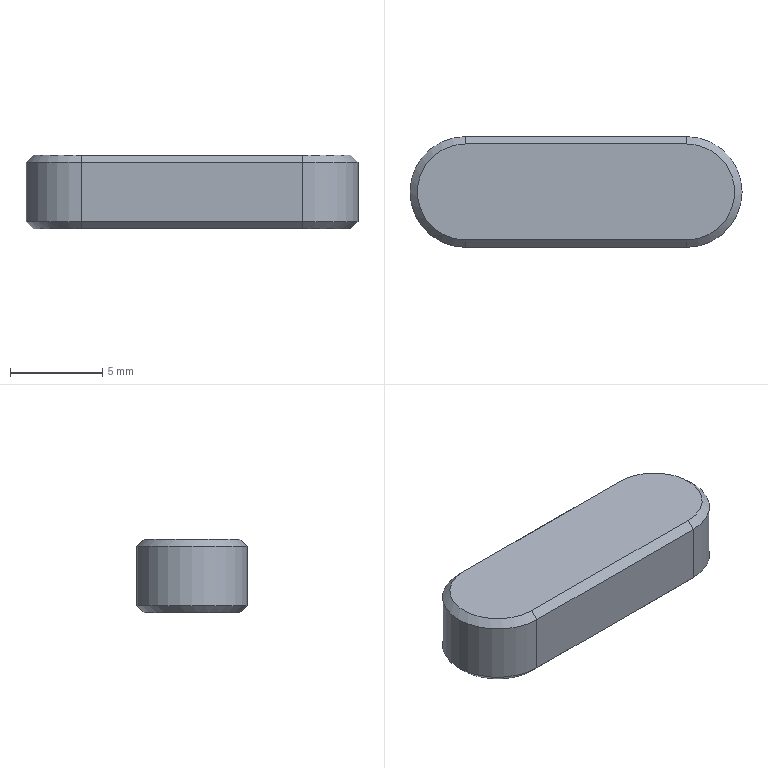Part | SolidWorks | features BaseBody 1 | 1 solid | 14 faces | box 18 x 6 x 4 mm | volume 394.375 mm3 | plane 8 | cone 4 | cylinder 2 | commonest cylinder face diameters 6 x2
STEP:
#1=CARTESIAN_POINT('',(15.,-2.6,-2.5));
#2=VERTEX_POINT('',#1);
#3=CARTESIAN_POINT('',(15.,-3.,-2.1));
#4=VERTEX_POINT('',#3);
#5=CARTESIAN_POINT('',(15.,-2.6,-2.5));
#6=DIRECTION('',(0.,-0.7071,0.7071));
#7=VECTOR('',#6,1000.);
#8=LINE('',#5,#7);
#9=EDGE_CURVE('',#2,#4,#8,.T.);
#10=ORIENTED_EDGE('',*,*,#9,.T.);
#11=CARTESIAN_POINT('',(3.,-3.,-2.1));
#12=VERTEX_POINT('',#11);
#13=CARTESIAN_POINT('',(6.,-3.,-2.1));
#14=DIRECTION('',(-1.,0.,0.));
#15=VECTOR('',#14,1000.);
#16=LINE('',#13,#15);
#17=EDGE_CURVE('',#4,#12,#16,.T.);
#18=ORIENTED_EDGE('',*,*,#17,.T.);
#19=CARTESIAN_POINT('',(3.,-2.6,-2.5));
#20=VERTEX_POINT('',#19);
#21=CARTESIAN_POINT('',(3.,-3.,-2.1));
#22=DIRECTION('',(0.,0.7071,-0.7071));
#23=VECTOR('',#22,1000.);
#24=LINE('',#21,#23);
#25=EDGE_CURVE('',#12,#20,#24,.T.);
#26=ORIENTED_EDGE('',*,*,#25,.T.);
#27=CARTESIAN_POINT('',(6.,-2.6,-2.5));
#28=DIRECTION('',(1.,0.,0.));
#29=VECTOR('',#28,1000.);
#30=LINE('',#27,#29);
#31=EDGE_CURVE('',#20,#2,#30,.T.);
#32=ORIENTED_EDGE('',*,*,#31,.T.);
#33=EDGE_LOOP('',(#10,#18,#26,#32));
#34=FACE_OUTER_BOUND('',#33,.T.);
#35=CARTESIAN_POINT('',(6.,-2.8,-2.3));
#36=DIRECTION('',(0.,-0.7071,-0.7071));
#37=DIRECTION('',(0.,-0.7071,0.7071));
#38=AXIS2_PLACEMENT_3D('',#35,#36,#37);
#39=PLANE('',#38);
#40=ADVANCED_FACE('',(#34),#39,.T.);
#41=CARTESIAN_POINT('',(15.,2.6,-2.5));
#42=VERTEX_POINT('',#41);
#43=CARTESIAN_POINT('',(15.,3.,-2.1));
#44=VERTEX_POINT('',#43);
#45=CARTESIAN_POINT('',(15.,2.6,-2.5));
#46=DIRECTION('',(0.,0.7071,0.7071));
#47=VECTOR('',#46,1000.);
#48=LINE('',#45,#47);
#49=EDGE_CURVE('',#42,#44,#48,.T.);
#50=ORIENTED_EDGE('',*,*,#49,.T.);
#51=CARTESIAN_POINT('',(15.,0.,-2.1));
#52=DIRECTION('',(0.,0.,-1.));
#53=DIRECTION('',(0.,1.,0.));
#54=AXIS2_PLACEMENT_3D('',#51,#52,#53);
#55=CIRCLE('',#54,3.);
#56=EDGE_CURVE('',#44,#4,#55,.T.);
#57=ORIENTED_EDGE('',*,*,#56,.T.);
#58=ORIENTED_EDGE('',*,*,#9,.F.);
#59=CARTESIAN_POINT('',(15.,0.,-2.5));
#60=DIRECTION('',(0.,0.,1.));
#61=DIRECTION('',(0.,1.,0.));
#62=AXIS2_PLACEMENT_3D('',#59,#60,#61);
#63=CIRCLE('',#62,2.6);
#64=EDGE_CURVE('',#2,#42,#63,.T.);
#65=ORIENTED_EDGE('',*,*,#64,.T.);
#66=EDGE_LOOP('',(#50,#57,#58,#65));
#67=FACE_OUTER_BOUND('',#66,.T.);
#68=CARTESIAN_POINT('',(15.,0.,-2.3));
#69=DIRECTION('',(0.,0.,1.));
#70=DIRECTION('',(0.,1.,0.));
#71=AXIS2_PLACEMENT_3D('',#68,#69,#70);
#72=CONICAL_SURFACE('',#71,2.8,0.7854);
#73=ADVANCED_FACE('',(#67),#72,.T.);
#74=CARTESIAN_POINT('',(3.,3.,-2.1));
#75=VERTEX_POINT('',#74);
#76=CARTESIAN_POINT('',(3.,2.6,-2.5));
#77=VERTEX_POINT('',#76);
#78=CARTESIAN_POINT('',(3.,3.,-2.1));
#79=DIRECTION('',(0.,-0.7071,-0.7071));
#80=VECTOR('',#79,1000.);
#81=LINE('',#78,#80);
#82=EDGE_CURVE('',#75,#77,#81,.T.);
#83=ORIENTED_EDGE('',*,*,#82,.T.);
#84=CARTESIAN_POINT('',(3.,0.,-2.5));
#85=DIRECTION('',(0.,0.,1.));
#86=DIRECTION('',(0.,-1.,0.));
#87=AXIS2_PLACEMENT_3D('',#84,#85,#86);
#88=CIRCLE('',#87,2.6);
#89=EDGE_CURVE('',#77,#20,#88,.T.);
#90=ORIENTED_EDGE('',*,*,#89,.T.);
#91=ORIENTED_EDGE('',*,*,#25,.F.);
#92=CARTESIAN_POINT('',(3.,0.,-2.1));
#93=DIRECTION('',(0.,0.,-1.));
#94=DIRECTION('',(0.,-1.,0.));
#95=AXIS2_PLACEMENT_3D('',#92,#93,#94);
#96=CIRCLE('',#95,3.);
#97=EDGE_CURVE('',#12,#75,#96,.T.);
#98=ORIENTED_EDGE('',*,*,#97,.T.);
#99=EDGE_LOOP('',(#83,#90,#91,#98));
#100=FACE_OUTER_BOUND('',#99,.T.);
#101=CARTESIAN_POINT('',(3.,0.,-2.3));
#102=DIRECTION('',(0.,0.,1.));
#103=DIRECTION('',(0.,-1.,0.));
#104=AXIS2_PLACEMENT_3D('',#101,#102,#103);
#105=CONICAL_SURFACE('',#104,2.8,0.7854);
#106=ADVANCED_FACE('',(#100),#105,.T.);
#107=ORIENTED_EDGE('',*,*,#49,.F.);
#108=CARTESIAN_POINT('',(12.,2.6,-2.5));
#109=DIRECTION('',(-1.,0.,0.));
#110=VECTOR('',#109,1000.);
#111=LINE('',#108,#110);
#112=EDGE_CURVE('',#42,#77,#111,.T.);
#113=ORIENTED_EDGE('',*,*,#112,.T.);
#114=ORIENTED_EDGE('',*,*,#82,.F.);
#115=CARTESIAN_POINT('',(12.,3.,-2.1));
#116=DIRECTION('',(1.,0.,0.));
#117=VECTOR('',#116,1000.);
#118=LINE('',#115,#117);
#119=EDGE_CURVE('',#75,#44,#118,.T.);
#120=ORIENTED_EDGE('',*,*,#119,.T.);
#121=EDGE_LOOP('',(#107,#113,#114,#120));
#122=FACE_OUTER_BOUND('',#121,.T.);
#123=CARTESIAN_POINT('',(12.,2.8,-2.3));
#124=DIRECTION('',(0.,0.7071,-0.7071));
#125=DIRECTION('',(-1.,0.,0.));
#126=AXIS2_PLACEMENT_3D('',#123,#124,#125);
#127=PLANE('',#126);
#128=ADVANCED_FACE('',(#122),#127,.T.);
#129=ORIENTED_EDGE('',*,*,#97,.F.);
#130=CARTESIAN_POINT('',(3.,-3.,1.1));
#131=VERTEX_POINT('',#130);
#132=CARTESIAN_POINT('',(3.,-3.,0.));
#133=DIRECTION('',(0.,0.,-1.));
#134=VECTOR('',#133,1000.);
#135=LINE('',#132,#134);
#136=EDGE_CURVE('',#131,#12,#135,.T.);
#137=ORIENTED_EDGE('',*,*,#136,.F.);
#138=CARTESIAN_POINT('',(3.,3.,1.1));
#139=VERTEX_POINT('',#138);
#140=CARTESIAN_POINT('',(3.,0.,1.1));
#141=DIRECTION('',(0.,0.,1.));
#142=DIRECTION('',(0.,-1.,0.));
#143=AXIS2_PLACEMENT_3D('',#140,#141,#142);
#144=CIRCLE('',#143,3.);
#145=EDGE_CURVE('',#139,#131,#144,.T.);
#146=ORIENTED_EDGE('',*,*,#145,.F.);
#147=CARTESIAN_POINT('',(3.,3.,0.));
#148=DIRECTION('',(0.,0.,1.));
#149=VECTOR('',#148,1000.);
#150=LINE('',#147,#149);
#151=EDGE_CURVE('',#75,#139,#150,.T.);
#152=ORIENTED_EDGE('',*,*,#151,.F.);
#153=EDGE_LOOP('',(#129,#137,#146,#152));
#154=FACE_OUTER_BOUND('',#153,.T.);
#155=CARTESIAN_POINT('',(3.,0.,0.));
#156=DIRECTION('',(0.,0.,1.));
#157=DIRECTION('',(0.,-1.,0.));
#158=AXIS2_PLACEMENT_3D('',#155,#156,#157);
#159=CYLINDRICAL_SURFACE('',#158,3.);
#160=ADVANCED_FACE('',(#154),#159,.T.);
#161=ORIENTED_EDGE('',*,*,#17,.F.);
#162=CARTESIAN_POINT('',(15.,-3.,1.1));
#163=VERTEX_POINT('',#162);
#164=CARTESIAN_POINT('',(15.,-3.,0.));
#165=DIRECTION('',(0.,0.,-1.));
#166=VECTOR('',#165,1000.);
#167=LINE('',#164,#166);
#168=EDGE_CURVE('',#163,#4,#167,.T.);
#169=ORIENTED_EDGE('',*,*,#168,.F.);
#170=CARTESIAN_POINT('',(6.,-3.,1.1));
#171=DIRECTION('',(1.,0.,0.));
#172=VECTOR('',#171,1000.);
#173=LINE('',#170,#172);
#174=EDGE_CURVE('',#131,#163,#173,.T.);
#175=ORIENTED_EDGE('',*,*,#174,.F.);
#176=ORIENTED_EDGE('',*,*,#136,.T.);
#177=EDGE_LOOP('',(#161,#169,#175,#176));
#178=FACE_OUTER_BOUND('',#177,.T.);
#179=CARTESIAN_POINT('',(3.,-3.,0.));
#180=DIRECTION('',(0.,-1.,0.));
#181=DIRECTION('',(0.,0.,-1.));
#182=AXIS2_PLACEMENT_3D('',#179,#180,#181);
#183=PLANE('',#182);
#184=ADVANCED_FACE('',(#178),#183,.T.);
#185=ORIENTED_EDGE('',*,*,#31,.F.);
#186=ORIENTED_EDGE('',*,*,#89,.F.);
#187=ORIENTED_EDGE('',*,*,#112,.F.);
#188=ORIENTED_EDGE('',*,*,#64,.F.);
#189=EDGE_LOOP('',(#185,#186,#187,#188));
#190=FACE_OUTER_BOUND('',#189,.T.);
#191=CARTESIAN_POINT('',(9.,0.,-2.5));
#192=DIRECTION('',(0.,0.,1.));
#193=DIRECTION('',(1.,0.,0.));
#194=AXIS2_PLACEMENT_3D('',#191,#192,#193);
#195=PLANE('',#194);
#196=ADVANCED_FACE('',(#190),#195,.F.);
#197=CARTESIAN_POINT('',(3.,-2.6,1.5));
#198=VERTEX_POINT('',#197);
#199=CARTESIAN_POINT('',(3.,-3.,1.1));
#200=DIRECTION('',(0.,0.7071,0.7071));
#201=VECTOR('',#200,1000.);
#202=LINE('',#199,#201);
#203=EDGE_CURVE('',#131,#198,#202,.T.);
#204=ORIENTED_EDGE('',*,*,#203,.T.);
#205=CARTESIAN_POINT('',(3.,2.6,1.5));
#206=VERTEX_POINT('',#205);
#207=CARTESIAN_POINT('',(3.,0.,1.5));
#208=DIRECTION('',(0.,0.,-1.));
#209=DIRECTION('',(0.,-1.,0.));
#210=AXIS2_PLACEMENT_3D('',#207,#208,#209);
#211=CIRCLE('',#210,2.6);
#212=EDGE_CURVE('',#198,#206,#211,.T.);
#213=ORIENTED_EDGE('',*,*,#212,.T.);
#214=CARTESIAN_POINT('',(3.,2.6,1.5));
#215=DIRECTION('',(0.,0.7071,-0.7071));
#216=VECTOR('',#215,1000.);
#217=LINE('',#214,#216);
#218=EDGE_CURVE('',#206,#139,#217,.T.);
#219=ORIENTED_EDGE('',*,*,#218,.T.);
#220=ORIENTED_EDGE('',*,*,#145,.T.);
#221=EDGE_LOOP('',(#204,#213,#219,#220));
#222=FACE_OUTER_BOUND('',#221,.T.);
#223=CARTESIAN_POINT('',(3.,0.,1.3));
#224=DIRECTION('',(0.,0.,-1.));
#225=DIRECTION('',(0.,-1.,0.));
#226=AXIS2_PLACEMENT_3D('',#223,#224,#225);
#227=CONICAL_SURFACE('',#226,2.8,0.7854);
#228=ADVANCED_FACE('',(#222),#227,.T.);
#229=CARTESIAN_POINT('',(15.,-2.6,1.5));
#230=VERTEX_POINT('',#229);
#231=CARTESIAN_POINT('',(15.,-3.,1.1));
#232=DIRECTION('',(0.,0.7071,0.7071));
#233=VECTOR('',#232,1000.);
#234=LINE('',#231,#233);
#235=EDGE_CURVE('',#163,#230,#234,.T.);
#236=ORIENTED_EDGE('',*,*,#235,.T.);
#237=CARTESIAN_POINT('',(6.,-2.6,1.5));
#238=DIRECTION('',(-1.,0.,0.));
#239=VECTOR('',#238,1000.);
#240=LINE('',#237,#239);
#241=EDGE_CURVE('',#230,#198,#240,.T.);
#242=ORIENTED_EDGE('',*,*,#241,.T.);
#243=ORIENTED_EDGE('',*,*,#203,.F.);
#244=ORIENTED_EDGE('',*,*,#174,.T.);
#245=EDGE_LOOP('',(#236,#242,#243,#244));
#246=FACE_OUTER_BOUND('',#245,.T.);
#247=CARTESIAN_POINT('',(6.,-2.8,1.3));
#248=DIRECTION('',(0.,-0.7071,0.7071));
#249=DIRECTION('',(-1.,0.,0.));
#250=AXIS2_PLACEMENT_3D('',#247,#248,#249);
#251=PLANE('',#250);
#252=ADVANCED_FACE('',(#246),#251,.T.);
#253=CARTESIAN_POINT('',(15.,2.6,1.5));
#254=VERTEX_POINT('',#253);
#255=CARTESIAN_POINT('',(15.,3.,1.1));
#256=VERTEX_POINT('',#255);
#257=CARTESIAN_POINT('',(15.,2.6,1.5));
#258=DIRECTION('',(0.,0.7071,-0.7071));
#259=VECTOR('',#258,1000.);
#260=LINE('',#257,#259);
#261=EDGE_CURVE('',#254,#256,#260,.T.);
#262=ORIENTED_EDGE('',*,*,#261,.T.);
#263=CARTESIAN_POINT('',(12.,3.,1.1));
#264=DIRECTION('',(-1.,0.,0.));
#265=VECTOR('',#264,1000.);
#266=LINE('',#263,#265);
#267=EDGE_CURVE('',#256,#139,#266,.T.);
#268=ORIENTED_EDGE('',*,*,#267,.T.);
#269=ORIENTED_EDGE('',*,*,#218,.F.);
#270=CARTESIAN_POINT('',(12.,2.6,1.5));
#271=DIRECTION('',(1.,0.,0.));
#272=VECTOR('',#271,1000.);
#273=LINE('',#270,#272);
#274=EDGE_CURVE('',#206,#254,#273,.T.);
#275=ORIENTED_EDGE('',*,*,#274,.T.);
#276=EDGE_LOOP('',(#262,#268,#269,#275));
#277=FACE_OUTER_BOUND('',#276,.T.);
#278=CARTESIAN_POINT('',(12.,2.8,1.3));
#279=DIRECTION('',(0.,0.7071,0.7071));
#280=DIRECTION('',(1.,0.,0.));
#281=AXIS2_PLACEMENT_3D('',#278,#279,#280);
#282=PLANE('',#281);
#283=ADVANCED_FACE('',(#277),#282,.T.);
#284=ORIENTED_EDGE('',*,*,#235,.F.);
#285=CARTESIAN_POINT('',(15.,0.,1.1));
#286=DIRECTION('',(0.,0.,1.));
#287=DIRECTION('',(0.,1.,0.));
#288=AXIS2_PLACEMENT_3D('',#285,#286,#287);
#289=CIRCLE('',#288,3.);
#290=EDGE_CURVE('',#163,#256,#289,.T.);
#291=ORIENTED_EDGE('',*,*,#290,.T.);
#292=ORIENTED_EDGE('',*,*,#261,.F.);
#293=CARTESIAN_POINT('',(15.,0.,1.5));
#294=DIRECTION('',(0.,0.,-1.));
#295=DIRECTION('',(0.,1.,0.));
#296=AXIS2_PLACEMENT_3D('',#293,#294,#295);
#297=CIRCLE('',#296,2.6);
#298=EDGE_CURVE('',#254,#230,#297,.T.);
#299=ORIENTED_EDGE('',*,*,#298,.T.);
#300=EDGE_LOOP('',(#284,#291,#292,#299));
#301=FACE_OUTER_BOUND('',#300,.T.);
#302=CARTESIAN_POINT('',(15.,0.,1.3));
#303=DIRECTION('',(0.,0.,-1.));
#304=DIRECTION('',(0.,1.,0.));
#305=AXIS2_PLACEMENT_3D('',#302,#303,#304);
#306=CONICAL_SURFACE('',#305,2.8,0.7854);
#307=ADVANCED_FACE('',(#301),#306,.T.);
#308=ORIENTED_EDGE('',*,*,#212,.F.);
#309=ORIENTED_EDGE('',*,*,#241,.F.);
#310=ORIENTED_EDGE('',*,*,#298,.F.);
#311=ORIENTED_EDGE('',*,*,#274,.F.);
#312=EDGE_LOOP('',(#308,#309,#310,#311));
#313=FACE_OUTER_BOUND('',#312,.T.);
#314=CARTESIAN_POINT('',(9.,0.,1.5));
#315=DIRECTION('',(0.,0.,1.));
#316=DIRECTION('',(1.,0.,0.));
#317=AXIS2_PLACEMENT_3D('',#314,#315,#316);
#318=PLANE('',#317);
#319=ADVANCED_FACE('',(#313),#318,.T.);
#320=ORIENTED_EDGE('',*,*,#119,.F.);
#321=ORIENTED_EDGE('',*,*,#151,.T.);
#322=ORIENTED_EDGE('',*,*,#267,.F.);
#323=CARTESIAN_POINT('',(15.,3.,0.));
#324=DIRECTION('',(0.,0.,-1.));
#325=VECTOR('',#324,1000.);
#326=LINE('',#323,#325);
#327=EDGE_CURVE('',#256,#44,#326,.T.);
#328=ORIENTED_EDGE('',*,*,#327,.T.);
#329=EDGE_LOOP('',(#320,#321,#322,#328));
#330=FACE_OUTER_BOUND('',#329,.T.);
#331=CARTESIAN_POINT('',(15.,3.,0.));
#332=DIRECTION('',(0.,1.,0.));
#333=DIRECTION('',(1.,0.,0.));
#334=AXIS2_PLACEMENT_3D('',#331,#332,#333);
#335=PLANE('',#334);
#336=ADVANCED_FACE('',(#330),#335,.T.);
#337=ORIENTED_EDGE('',*,*,#56,.F.);
#338=ORIENTED_EDGE('',*,*,#327,.F.);
#339=ORIENTED_EDGE('',*,*,#290,.F.);
#340=ORIENTED_EDGE('',*,*,#168,.T.);
#341=EDGE_LOOP('',(#337,#338,#339,#340));
#342=FACE_OUTER_BOUND('',#341,.T.);
#343=CARTESIAN_POINT('',(15.,0.,0.));
#344=DIRECTION('',(0.,0.,1.));
#345=DIRECTION('',(0.,1.,0.));
#346=AXIS2_PLACEMENT_3D('',#343,#344,#345);
#347=CYLINDRICAL_SURFACE('',#346,3.);
#348=ADVANCED_FACE('',(#342),#347,.T.);
#349=CLOSED_SHELL('',(#40,#73,#106,#128,#160,#184,#196,#228,#252,#283,#307,#319,#336,#348));
#350=MANIFOLD_SOLID_BREP('',#349);
#351=CARTESIAN_POINT('',(0.,0.,0.));
#352=DIRECTION('',(0.,0.,1.));
#353=DIRECTION('',(1.,0.,0.));
#354=AXIS2_PLACEMENT_3D('',#351,#352,#353);
#355=(LENGTH_UNIT()NAMED_UNIT(*)SI_UNIT(.MILLI.,.METRE.));
#356=UNCERTAINTY_MEASURE_WITH_UNIT(LENGTH_MEASURE(0.00001),#355,'','');
#357=(NAMED_UNIT(*)PLANE_ANGLE_UNIT()SI_UNIT($,.RADIAN.));
#358=(NAMED_UNIT(*)SI_UNIT($,.STERADIAN.)SOLID_ANGLE_UNIT());
#359=(GEOMETRIC_REPRESENTATION_CONTEXT(3)GLOBAL_UNCERTAINTY_ASSIGNED_CONTEXT((#356))GLOBAL_UNIT_ASSIGNED_CONTEXT((#355,#357,#358))REPRESENTATION_CONTEXT('',''));
#360=ADVANCED_BREP_SHAPE_REPRESENTATION('',(#350,#354),#359);